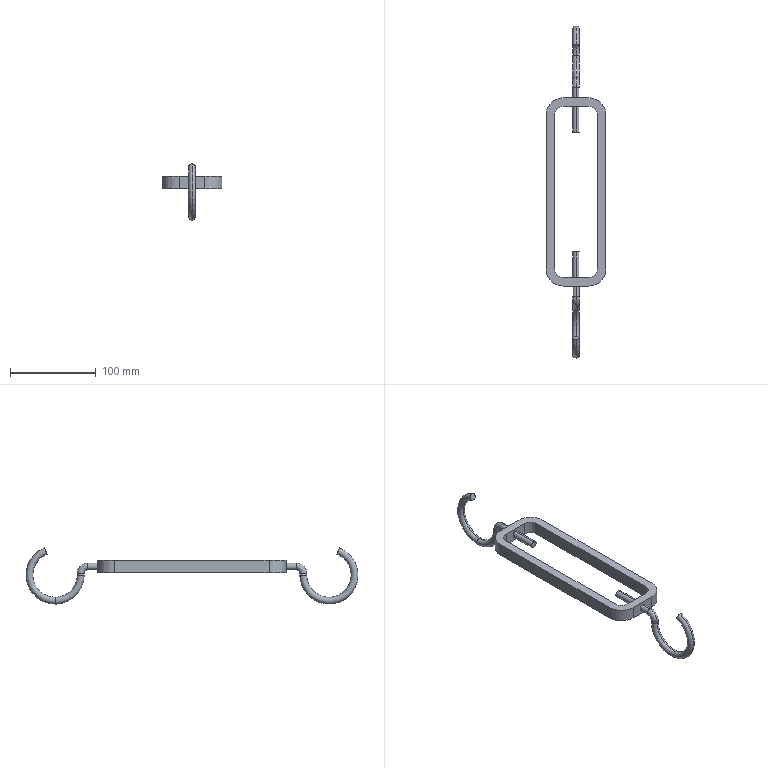Part | SolidWorks | features Extrusion 1, ICE 1, MirrorPattern 1, Sweep 1 | 1 solid | 44 faces | box 70 x 388 x 65.733 mm | volume 95929 mm3 | cylinder 20 | plane 14 | torus 10 | commonest cylinder face diameters 8 x12 20 x4 40 x4
STEP:
#1=CARTESIAN_POINT('',(-4.,-130.,-10.));
#2=VERTEX_POINT('',#1);
#3=CARTESIAN_POINT('',(0.,-126.,-10.));
#4=VERTEX_POINT('',#3);
#5=CARTESIAN_POINT('',(0.,-130.,-10.));
#6=DIRECTION('',(0.,0.,-1.));
#7=DIRECTION('',(0.,-1.,0.));
#8=AXIS2_PLACEMENT_3D('',#5,#6,#7);
#9=CIRCLE('',#8,4.);
#10=EDGE_CURVE('',#2,#4,#9,.T.);
#11=ORIENTED_EDGE('',*,*,#10,.T.);
#12=CARTESIAN_POINT('',(0.,-172.206,21.733));
#13=VERTEX_POINT('',#12);
#14=CARTESIAN_POINT('',(0.,-160.,-10.));
#15=DIRECTION('',(-1.,0.,0.));
#16=DIRECTION('',(0.,0.,1.));
#17=AXIS2_PLACEMENT_3D('',#14,#15,#16);
#18=CIRCLE('',#17,34.);
#19=EDGE_CURVE('',#4,#13,#18,.T.);
#20=ORIENTED_EDGE('',*,*,#19,.T.);
#21=CARTESIAN_POINT('',(0.,-169.334,14.267));
#22=VERTEX_POINT('',#21);
#23=CARTESIAN_POINT('',(0.,-170.77,18.));
#24=DIRECTION('',(0.,0.9333,0.359));
#25=DIRECTION('',(0.,0.359,-0.9333));
#26=AXIS2_PLACEMENT_3D('',#23,#24,#25);
#27=CIRCLE('',#26,4.);
#28=EDGE_CURVE('',#22,#13,#27,.T.);
#29=ORIENTED_EDGE('',*,*,#28,.F.);
#30=CARTESIAN_POINT('',(0.,-134.,-10.));
#31=VERTEX_POINT('',#30);
#32=CARTESIAN_POINT('',(0.,-160.,-10.));
#33=DIRECTION('',(-1.,0.,0.));
#34=DIRECTION('',(0.,0.,1.));
#35=AXIS2_PLACEMENT_3D('',#32,#33,#34);
#36=CIRCLE('',#35,26.);
#37=EDGE_CURVE('',#31,#22,#36,.T.);
#38=ORIENTED_EDGE('',*,*,#37,.F.);
#39=CARTESIAN_POINT('',(0.,-130.,-10.));
#40=DIRECTION('',(0.,0.,-1.));
#41=DIRECTION('',(0.,-1.,0.));
#42=AXIS2_PLACEMENT_3D('',#39,#40,#41);
#43=CIRCLE('',#42,4.);
#44=EDGE_CURVE('',#31,#2,#43,.T.);
#45=ORIENTED_EDGE('',*,*,#44,.T.);
#46=EDGE_LOOP('',(#11,#20,#29,#38,#45));
#47=FACE_OUTER_BOUND('',#46,.T.);
#48=CARTESIAN_POINT('',(0.,-160.,-10.));
#49=DIRECTION('',(-1.,0.,0.));
#50=DIRECTION('',(0.,0.,1.));
#51=AXIS2_PLACEMENT_3D('',#48,#49,#50);
#52=TOROIDAL_SURFACE('',#51,30.,4.);
#53=ADVANCED_FACE('',(#47),#52,.T.);
#54=CARTESIAN_POINT('',(0.,-122.,-4.));
#55=VERTEX_POINT('',#54);
#56=CARTESIAN_POINT('',(0.,-122.,4.));
#57=VERTEX_POINT('',#56);
#58=CARTESIAN_POINT('',(0.,-122.,0.));
#59=DIRECTION('',(0.,-1.,0.));
#60=DIRECTION('',(0.,0.,1.));
#61=AXIS2_PLACEMENT_3D('',#58,#59,#60);
#62=CIRCLE('',#61,4.);
#63=EDGE_CURVE('',#55,#57,#62,.T.);
#64=ORIENTED_EDGE('',*,*,#63,.T.);
#65=CARTESIAN_POINT('',(0.,-134.,-8.));
#66=VERTEX_POINT('',#65);
#67=CARTESIAN_POINT('',(0.,-122.,-8.));
#68=DIRECTION('',(1.,0.,0.));
#69=DIRECTION('',(0.,0.,-1.));
#70=AXIS2_PLACEMENT_3D('',#67,#68,#69);
#71=CIRCLE('',#70,12.);
#72=EDGE_CURVE('',#57,#66,#71,.T.);
#73=ORIENTED_EDGE('',*,*,#72,.T.);
#74=CARTESIAN_POINT('',(4.,-130.,-8.));
#75=VERTEX_POINT('',#74);
#76=CARTESIAN_POINT('',(0.,-130.,-8.));
#77=DIRECTION('',(0.,0.,-1.));
#78=DIRECTION('',(0.,-1.,0.));
#79=AXIS2_PLACEMENT_3D('',#76,#77,#78);
#80=CIRCLE('',#79,4.);
#81=EDGE_CURVE('',#75,#66,#80,.T.);
#82=ORIENTED_EDGE('',*,*,#81,.F.);
#83=CARTESIAN_POINT('',(0.,-126.,-8.));
#84=VERTEX_POINT('',#83);
#85=CARTESIAN_POINT('',(0.,-130.,-8.));
#86=DIRECTION('',(0.,0.,-1.));
#87=DIRECTION('',(0.,-1.,0.));
#88=AXIS2_PLACEMENT_3D('',#85,#86,#87);
#89=CIRCLE('',#88,4.);
#90=EDGE_CURVE('',#84,#75,#89,.T.);
#91=ORIENTED_EDGE('',*,*,#90,.F.);
#92=CARTESIAN_POINT('',(0.,-122.,-8.));
#93=DIRECTION('',(1.,0.,0.));
#94=DIRECTION('',(0.,0.,-1.));
#95=AXIS2_PLACEMENT_3D('',#92,#93,#94);
#96=CIRCLE('',#95,4.);
#97=EDGE_CURVE('',#55,#84,#96,.T.);
#98=ORIENTED_EDGE('',*,*,#97,.F.);
#99=EDGE_LOOP('',(#64,#73,#82,#91,#98));
#100=FACE_OUTER_BOUND('',#99,.T.);
#101=CARTESIAN_POINT('',(0.,-122.,-8.));
#102=DIRECTION('',(1.,0.,0.));
#103=DIRECTION('',(0.,0.,-1.));
#104=AXIS2_PLACEMENT_3D('',#101,#102,#103);
#105=TOROIDAL_SURFACE('',#104,8.,4.);
#106=ADVANCED_FACE('',(#100),#105,.T.);
#107=CARTESIAN_POINT('',(0.,160.,-44.));
#108=VERTEX_POINT('',#107);
#109=CARTESIAN_POINT('',(0.,160.,-36.));
#110=VERTEX_POINT('',#109);
#111=CARTESIAN_POINT('',(0.,160.,-40.));
#112=DIRECTION('',(0.,-1.,0.));
#113=DIRECTION('',(0.,0.,-1.));
#114=AXIS2_PLACEMENT_3D('',#111,#112,#113);
#115=CIRCLE('',#114,4.);
#116=EDGE_CURVE('',#108,#110,#115,.T.);
#117=ORIENTED_EDGE('',*,*,#116,.F.);
#118=CARTESIAN_POINT('',(0.,172.206,21.733));
#119=VERTEX_POINT('',#118);
#120=CARTESIAN_POINT('',(0.,160.,-10.));
#121=DIRECTION('',(1.,0.,0.));
#122=DIRECTION('',(0.,0.,-1.));
#123=AXIS2_PLACEMENT_3D('',#120,#121,#122);
#124=CIRCLE('',#123,34.);
#125=EDGE_CURVE('',#108,#119,#124,.T.);
#126=ORIENTED_EDGE('',*,*,#125,.T.);
#127=CARTESIAN_POINT('',(0.,169.334,14.267));
#128=VERTEX_POINT('',#127);
#129=CARTESIAN_POINT('',(0.,170.77,18.));
#130=DIRECTION('',(0.,-0.9333,0.359));
#131=DIRECTION('',(0.,-0.359,-0.9333));
#132=AXIS2_PLACEMENT_3D('',#129,#130,#131);
#133=CIRCLE('',#132,4.);
#134=EDGE_CURVE('',#128,#119,#133,.T.);
#135=ORIENTED_EDGE('',*,*,#134,.F.);
#136=CARTESIAN_POINT('',(0.,160.,-10.));
#137=DIRECTION('',(1.,0.,0.));
#138=DIRECTION('',(0.,0.,-1.));
#139=AXIS2_PLACEMENT_3D('',#136,#137,#138);
#140=CIRCLE('',#139,26.);
#141=EDGE_CURVE('',#110,#128,#140,.T.);
#142=ORIENTED_EDGE('',*,*,#141,.F.);
#143=EDGE_LOOP('',(#117,#126,#135,#142));
#144=FACE_OUTER_BOUND('',#143,.T.);
#145=CARTESIAN_POINT('',(0.,160.,-10.));
#146=DIRECTION('',(1.,0.,0.));
#147=DIRECTION('',(0.,0.,-1.));
#148=AXIS2_PLACEMENT_3D('',#145,#146,#147);
#149=TOROIDAL_SURFACE('',#148,30.,4.);
#150=ADVANCED_FACE('',(#144),#149,.T.);
#151=CARTESIAN_POINT('',(0.,122.,-4.));
#152=VERTEX_POINT('',#151);
#153=CARTESIAN_POINT('',(0.,122.,4.));
#154=VERTEX_POINT('',#153);
#155=CARTESIAN_POINT('',(0.,122.,0.));
#156=DIRECTION('',(0.,1.,0.));
#157=DIRECTION('',(0.,0.,1.));
#158=AXIS2_PLACEMENT_3D('',#155,#156,#157);
#159=CIRCLE('',#158,4.);
#160=EDGE_CURVE('',#152,#154,#159,.T.);
#161=ORIENTED_EDGE('',*,*,#160,.T.);
#162=CARTESIAN_POINT('',(0.,134.,-8.));
#163=VERTEX_POINT('',#162);
#164=CARTESIAN_POINT('',(0.,122.,-8.));
#165=DIRECTION('',(-1.,0.,0.));
#166=DIRECTION('',(0.,0.,1.));
#167=AXIS2_PLACEMENT_3D('',#164,#165,#166);
#168=CIRCLE('',#167,12.);
#169=EDGE_CURVE('',#154,#163,#168,.T.);
#170=ORIENTED_EDGE('',*,*,#169,.T.);
#171=CARTESIAN_POINT('',(-4.,130.,-8.));
#172=VERTEX_POINT('',#171);
#173=CARTESIAN_POINT('',(0.,130.,-8.));
#174=DIRECTION('',(0.,0.,-1.));
#175=DIRECTION('',(0.,1.,0.));
#176=AXIS2_PLACEMENT_3D('',#173,#174,#175);
#177=CIRCLE('',#176,4.);
#178=EDGE_CURVE('',#172,#163,#177,.T.);
#179=ORIENTED_EDGE('',*,*,#178,.F.);
#180=CARTESIAN_POINT('',(0.,126.,-8.));
#181=VERTEX_POINT('',#180);
#182=CARTESIAN_POINT('',(0.,130.,-8.));
#183=DIRECTION('',(0.,0.,-1.));
#184=DIRECTION('',(0.,1.,0.));
#185=AXIS2_PLACEMENT_3D('',#182,#183,#184);
#186=CIRCLE('',#185,4.);
#187=EDGE_CURVE('',#181,#172,#186,.T.);
#188=ORIENTED_EDGE('',*,*,#187,.F.);
#189=CARTESIAN_POINT('',(0.,122.,-8.));
#190=DIRECTION('',(-1.,0.,0.));
#191=DIRECTION('',(0.,0.,1.));
#192=AXIS2_PLACEMENT_3D('',#189,#190,#191);
#193=CIRCLE('',#192,4.);
#194=EDGE_CURVE('',#152,#181,#193,.T.);
#195=ORIENTED_EDGE('',*,*,#194,.F.);
#196=EDGE_LOOP('',(#161,#170,#179,#188,#195));
#197=FACE_OUTER_BOUND('',#196,.T.);
#198=CARTESIAN_POINT('',(0.,122.,-8.));
#199=DIRECTION('',(-1.,0.,0.));
#200=DIRECTION('',(0.,0.,1.));
#201=AXIS2_PLACEMENT_3D('',#198,#199,#200);
#202=TOROIDAL_SURFACE('',#201,8.,4.);
#203=ADVANCED_FACE('',(#197),#202,.T.);
#204=CARTESIAN_POINT('',(4.,130.,-10.));
#205=VERTEX_POINT('',#204);
#206=CARTESIAN_POINT('',(0.,126.,-10.));
#207=VERTEX_POINT('',#206);
#208=CARTESIAN_POINT('',(0.,130.,-10.));
#209=DIRECTION('',(0.,0.,-1.));
#210=DIRECTION('',(0.,1.,0.));
#211=AXIS2_PLACEMENT_3D('',#208,#209,#210);
#212=CIRCLE('',#211,4.);
#213=EDGE_CURVE('',#205,#207,#212,.T.);
#214=ORIENTED_EDGE('',*,*,#213,.T.);
#215=CARTESIAN_POINT('',(0.,160.,-10.));
#216=DIRECTION('',(1.,0.,0.));
#217=DIRECTION('',(0.,0.,-1.));
#218=AXIS2_PLACEMENT_3D('',#215,#216,#217);
#219=CIRCLE('',#218,34.);
#220=EDGE_CURVE('',#207,#108,#219,.T.);
#221=ORIENTED_EDGE('',*,*,#220,.T.);
#222=ORIENTED_EDGE('',*,*,#116,.T.);
#223=CARTESIAN_POINT('',(0.,134.,-10.));
#224=VERTEX_POINT('',#223);
#225=CARTESIAN_POINT('',(0.,160.,-10.));
#226=DIRECTION('',(1.,0.,0.));
#227=DIRECTION('',(0.,0.,-1.));
#228=AXIS2_PLACEMENT_3D('',#225,#226,#227);
#229=CIRCLE('',#228,26.);
#230=EDGE_CURVE('',#224,#110,#229,.T.);
#231=ORIENTED_EDGE('',*,*,#230,.F.);
#232=CARTESIAN_POINT('',(0.,130.,-10.));
#233=DIRECTION('',(0.,0.,-1.));
#234=DIRECTION('',(0.,1.,0.));
#235=AXIS2_PLACEMENT_3D('',#232,#233,#234);
#236=CIRCLE('',#235,4.);
#237=EDGE_CURVE('',#224,#205,#236,.T.);
#238=ORIENTED_EDGE('',*,*,#237,.T.);
#239=EDGE_LOOP('',(#214,#221,#222,#231,#238));
#240=FACE_OUTER_BOUND('',#239,.T.);
#241=CARTESIAN_POINT('',(0.,160.,-10.));
#242=DIRECTION('',(1.,0.,0.));
#243=DIRECTION('',(0.,0.,-1.));
#244=AXIS2_PLACEMENT_3D('',#241,#242,#243);
#245=TOROIDAL_SURFACE('',#244,30.,4.);
#246=ADVANCED_FACE('',(#240),#245,.T.);
#247=CARTESIAN_POINT('',(0.,-70.,-4.));
#248=VERTEX_POINT('',#247);
#249=CARTESIAN_POINT('',(0.,-70.,4.));
#250=VERTEX_POINT('',#249);
#251=CARTESIAN_POINT('',(0.,-70.,0.));
#252=DIRECTION('',(0.,-1.,0.));
#253=DIRECTION('',(0.,0.,-1.));
#254=AXIS2_PLACEMENT_3D('',#251,#252,#253);
#255=CIRCLE('',#254,4.);
#256=EDGE_CURVE('',#248,#250,#255,.T.);
#257=ORIENTED_EDGE('',*,*,#256,.T.);
#258=CARTESIAN_POINT('',(0.,-100.,4.));
#259=VERTEX_POINT('',#258);
#260=CARTESIAN_POINT('',(0.,-70.,4.));
#261=DIRECTION('',(0.,-1.,0.));
#262=VECTOR('',#261,1000.);
#263=LINE('',#260,#262);
#264=EDGE_CURVE('',#250,#259,#263,.T.);
#265=ORIENTED_EDGE('',*,*,#264,.T.);
#266=CARTESIAN_POINT('',(0.,-100.,-4.));
#267=VERTEX_POINT('',#266);
#268=CARTESIAN_POINT('',(0.,-100.,0.));
#269=DIRECTION('',(0.,1.,0.));
#270=DIRECTION('',(0.,0.,1.));
#271=AXIS2_PLACEMENT_3D('',#268,#269,#270);
#272=CIRCLE('',#271,4.);
#273=EDGE_CURVE('',#259,#267,#272,.T.);
#274=ORIENTED_EDGE('',*,*,#273,.T.);
#275=CARTESIAN_POINT('',(0.,-70.,-4.));
#276=DIRECTION('',(0.,-1.,0.));
#277=VECTOR('',#276,1000.);
#278=LINE('',#275,#277);
#279=EDGE_CURVE('',#248,#267,#278,.T.);
#280=ORIENTED_EDGE('',*,*,#279,.F.);
#281=EDGE_LOOP('',(#257,#265,#274,#280));
#282=FACE_OUTER_BOUND('',#281,.T.);
#283=CARTESIAN_POINT('',(0.,-70.,0.));
#284=DIRECTION('',(0.,-1.,0.));
#285=DIRECTION('',(0.,0.,-1.));
#286=AXIS2_PLACEMENT_3D('',#283,#284,#285);
#287=CYLINDRICAL_SURFACE('',#286,4.);
#288=ADVANCED_FACE('',(#282),#287,.T.);
#289=CARTESIAN_POINT('',(-4.,-130.,-8.));
#290=VERTEX_POINT('',#289);
#291=CARTESIAN_POINT('',(0.,-130.,-8.));
#292=DIRECTION('',(0.,0.,-1.));
#293=DIRECTION('',(0.,-1.,0.));
#294=AXIS2_PLACEMENT_3D('',#291,#292,#293);
#295=CIRCLE('',#294,4.);
#296=EDGE_CURVE('',#290,#84,#295,.T.);
#297=ORIENTED_EDGE('',*,*,#296,.T.);
#298=ORIENTED_EDGE('',*,*,#90,.T.);
#299=CARTESIAN_POINT('',(4.,-130.,-10.));
#300=VERTEX_POINT('',#299);
#301=CARTESIAN_POINT('',(4.,-130.,-8.));
#302=DIRECTION('',(0.,0.,-1.));
#303=VECTOR('',#302,1000.);
#304=LINE('',#301,#303);
#305=EDGE_CURVE('',#75,#300,#304,.T.);
#306=ORIENTED_EDGE('',*,*,#305,.T.);
#307=CARTESIAN_POINT('',(0.,-130.,-10.));
#308=DIRECTION('',(0.,0.,-1.));
#309=DIRECTION('',(0.,-1.,0.));
#310=AXIS2_PLACEMENT_3D('',#307,#308,#309);
#311=CIRCLE('',#310,4.);
#312=EDGE_CURVE('',#4,#300,#311,.T.);
#313=ORIENTED_EDGE('',*,*,#312,.F.);
#314=ORIENTED_EDGE('',*,*,#10,.F.);
#315=CARTESIAN_POINT('',(-4.,-130.,-8.));
#316=DIRECTION('',(0.,0.,-1.));
#317=VECTOR('',#316,1000.);
#318=LINE('',#315,#317);
#319=EDGE_CURVE('',#290,#2,#318,.T.);
#320=ORIENTED_EDGE('',*,*,#319,.F.);
#321=EDGE_LOOP('',(#297,#298,#306,#313,#314,#320));
#322=FACE_OUTER_BOUND('',#321,.T.);
#323=CARTESIAN_POINT('',(0.,-130.,-8.));
#324=DIRECTION('',(0.,0.,-1.));
#325=DIRECTION('',(-1.,0.,0.));
#326=AXIS2_PLACEMENT_3D('',#323,#324,#325);
#327=CYLINDRICAL_SURFACE('',#326,4.);
#328=ADVANCED_FACE('',(#322),#327,.T.);
#329=CARTESIAN_POINT('',(0.,-110.,-4.));
#330=VERTEX_POINT('',#329);
#331=CARTESIAN_POINT('',(0.,-110.,4.));
#332=VERTEX_POINT('',#331);
#333=CARTESIAN_POINT('',(0.,-110.,0.));
#334=DIRECTION('',(0.,-1.,0.));
#335=DIRECTION('',(0.,0.,1.));
#336=AXIS2_PLACEMENT_3D('',#333,#334,#335);
#337=CIRCLE('',#336,4.);
#338=EDGE_CURVE('',#330,#332,#337,.T.);
#339=ORIENTED_EDGE('',*,*,#338,.T.);
#340=CARTESIAN_POINT('',(0.,-110.,4.));
#341=DIRECTION('',(0.,-1.,0.));
#342=VECTOR('',#341,1000.);
#343=LINE('',#340,#342);
#344=EDGE_CURVE('',#332,#57,#343,.T.);
#345=ORIENTED_EDGE('',*,*,#344,.T.);
#346=ORIENTED_EDGE('',*,*,#63,.F.);
#347=CARTESIAN_POINT('',(0.,-110.,-4.));
#348=DIRECTION('',(0.,-1.,0.));
#349=VECTOR('',#348,1000.);
#350=LINE('',#347,#349);
#351=EDGE_CURVE('',#330,#55,#350,.T.);
#352=ORIENTED_EDGE('',*,*,#351,.F.);
#353=EDGE_LOOP('',(#339,#345,#346,#352));
#354=FACE_OUTER_BOUND('',#353,.T.);
#355=CARTESIAN_POINT('',(0.,-110.,0.));
#356=DIRECTION('',(0.,-1.,0.));
#357=DIRECTION('',(0.,0.,-1.));
#358=AXIS2_PLACEMENT_3D('',#355,#356,#357);
#359=CYLINDRICAL_SURFACE('',#358,4.);
#360=ADVANCED_FACE('',(#354),#359,.T.);
#361=CARTESIAN_POINT('',(0.,70.,-4.));
#362=VERTEX_POINT('',#361);
#363=CARTESIAN_POINT('',(0.,70.,4.));
#364=VERTEX_POINT('',#363);
#365=CARTESIAN_POINT('',(0.,70.,0.));
#366=DIRECTION('',(0.,-1.,0.));
#367=DIRECTION('',(0.,0.,-1.));
#368=AXIS2_PLACEMENT_3D('',#365,#366,#367);
#369=CIRCLE('',#368,4.);
#370=EDGE_CURVE('',#362,#364,#369,.T.);
#371=ORIENTED_EDGE('',*,*,#370,.F.);
#372=CARTESIAN_POINT('',(0.,100.,-4.));
#373=VERTEX_POINT('',#372);
#374=CARTESIAN_POINT('',(0.,70.,-4.));
#375=DIRECTION('',(0.,1.,0.));
#376=VECTOR('',#375,1000.);
#377=LINE('',#374,#376);
#378=EDGE_CURVE('',#362,#373,#377,.T.);
#379=ORIENTED_EDGE('',*,*,#378,.T.);
#380=CARTESIAN_POINT('',(0.,100.,4.));
#381=VERTEX_POINT('',#380);
#382=CARTESIAN_POINT('',(0.,100.,0.));
#383=DIRECTION('',(0.,-1.,0.));
#384=DIRECTION('',(0.,0.,-1.));
#385=AXIS2_PLACEMENT_3D('',#382,#383,#384);
#386=CIRCLE('',#385,4.);
#387=EDGE_CURVE('',#373,#381,#386,.T.);
#388=ORIENTED_EDGE('',*,*,#387,.T.);
#389=CARTESIAN_POINT('',(0.,70.,4.));
#390=DIRECTION('',(0.,1.,0.));
#391=VECTOR('',#390,1000.);
#392=LINE('',#389,#391);
#393=EDGE_CURVE('',#364,#381,#392,.T.);
#394=ORIENTED_EDGE('',*,*,#393,.F.);
#395=EDGE_LOOP('',(#371,#379,#388,#394));
#396=FACE_OUTER_BOUND('',#395,.T.);
#397=CARTESIAN_POINT('',(0.,70.,0.));
#398=DIRECTION('',(0.,1.,0.));
#399=DIRECTION('',(0.,0.,1.));
#400=AXIS2_PLACEMENT_3D('',#397,#398,#399);
#401=CYLINDRICAL_SURFACE('',#400,4.);
#402=ADVANCED_FACE('',(#396),#401,.T.);
#403=ORIENTED_EDGE('',*,*,#220,.F.);
#404=CARTESIAN_POINT('',(-4.,130.,-10.));
#405=VERTEX_POINT('',#404);
#406=CARTESIAN_POINT('',(0.,130.,-10.));
#407=DIRECTION('',(0.,0.,-1.));
#408=DIRECTION('',(0.,1.,0.));
#409=AXIS2_PLACEMENT_3D('',#406,#407,#408);
#410=CIRCLE('',#409,4.);
#411=EDGE_CURVE('',#207,#405,#410,.T.);
#412=ORIENTED_EDGE('',*,*,#411,.T.);
#413=CARTESIAN_POINT('',(0.,130.,-10.));
#414=DIRECTION('',(0.,0.,-1.));
#415=DIRECTION('',(0.,1.,0.));
#416=AXIS2_PLACEMENT_3D('',#413,#414,#415);
#417=CIRCLE('',#416,4.);
#418=EDGE_CURVE('',#405,#224,#417,.T.);
#419=ORIENTED_EDGE('',*,*,#418,.T.);
#420=ORIENTED_EDGE('',*,*,#230,.T.);
#421=CARTESIAN_POINT('',(0.,160.,-40.));
#422=DIRECTION('',(0.,-1.,0.));
#423=DIRECTION('',(0.,0.,-1.));
#424=AXIS2_PLACEMENT_3D('',#421,#422,#423);
#425=CIRCLE('',#424,4.);
#426=EDGE_CURVE('',#110,#108,#425,.T.);
#427=ORIENTED_EDGE('',*,*,#426,.T.);
#428=EDGE_LOOP('',(#403,#412,#419,#420,#427));
#429=FACE_OUTER_BOUND('',#428,.T.);
#430=CARTESIAN_POINT('',(0.,160.,-10.));
#431=DIRECTION('',(1.,0.,0.));
#432=DIRECTION('',(0.,0.,-1.));
#433=AXIS2_PLACEMENT_3D('',#430,#431,#432);
#434=TOROIDAL_SURFACE('',#433,30.,4.);
#435=ADVANCED_FACE('',(#429),#434,.T.);
#436=ORIENTED_EDGE('',*,*,#178,.T.);
#437=CARTESIAN_POINT('',(4.,130.,-8.));
#438=VERTEX_POINT('',#437);
#439=CARTESIAN_POINT('',(0.,130.,-8.));
#440=DIRECTION('',(0.,0.,-1.));
#441=DIRECTION('',(0.,1.,0.));
#442=AXIS2_PLACEMENT_3D('',#439,#440,#441);
#443=CIRCLE('',#442,4.);
#444=EDGE_CURVE('',#163,#438,#443,.T.);
#445=ORIENTED_EDGE('',*,*,#444,.T.);
#446=CARTESIAN_POINT('',(4.,130.,-8.));
#447=DIRECTION('',(0.,0.,-1.));
#448=VECTOR('',#447,1000.);
#449=LINE('',#446,#448);
#450=EDGE_CURVE('',#438,#205,#449,.T.);
#451=ORIENTED_EDGE('',*,*,#450,.T.);
#452=ORIENTED_EDGE('',*,*,#237,.F.);
#453=ORIENTED_EDGE('',*,*,#418,.F.);
#454=CARTESIAN_POINT('',(-4.,130.,-8.));
#455=DIRECTION('',(0.,0.,-1.));
#456=VECTOR('',#455,1000.);
#457=LINE('',#454,#456);
#458=EDGE_CURVE('',#172,#405,#457,.T.);
#459=ORIENTED_EDGE('',*,*,#458,.F.);
#460=EDGE_LOOP('',(#436,#445,#451,#452,#453,#459));
#461=FACE_OUTER_BOUND('',#460,.T.);
#462=CARTESIAN_POINT('',(0.,130.,-8.));
#463=DIRECTION('',(0.,0.,-1.));
#464=DIRECTION('',(-1.,0.,0.));
#465=AXIS2_PLACEMENT_3D('',#462,#463,#464);
#466=CYLINDRICAL_SURFACE('',#465,4.);
#467=ADVANCED_FACE('',(#461),#466,.T.);
#468=CARTESIAN_POINT('',(0.,110.,4.));
#469=VERTEX_POINT('',#468);
#470=CARTESIAN_POINT('',(0.,110.,-4.));
#471=VERTEX_POINT('',#470);
#472=CARTESIAN_POINT('',(0.,110.,0.));
#473=DIRECTION('',(0.,1.,0.));
#474=DIRECTION('',(0.,0.,1.));
#475=AXIS2_PLACEMENT_3D('',#472,#473,#474);
#476=CIRCLE('',#475,4.);
#477=EDGE_CURVE('',#469,#471,#476,.T.);
#478=ORIENTED_EDGE('',*,*,#477,.T.);
#479=CARTESIAN_POINT('',(0.,110.,-4.));
#480=DIRECTION('',(0.,1.,0.));
#481=VECTOR('',#480,1000.);
#482=LINE('',#479,#481);
#483=EDGE_CURVE('',#471,#152,#482,.T.);
#484=ORIENTED_EDGE('',*,*,#483,.T.);
#485=CARTESIAN_POINT('',(0.,122.,0.));
#486=DIRECTION('',(0.,1.,0.));
#487=DIRECTION('',(0.,0.,1.));
#488=AXIS2_PLACEMENT_3D('',#485,#486,#487);
#489=CIRCLE('',#488,4.);
#490=EDGE_CURVE('',#154,#152,#489,.T.);
#491=ORIENTED_EDGE('',*,*,#490,.F.);
#492=CARTESIAN_POINT('',(0.,110.,4.));
#493=DIRECTION('',(0.,1.,0.));
#494=VECTOR('',#493,1000.);
#495=LINE('',#492,#494);
#496=EDGE_CURVE('',#469,#154,#495,.T.);
#497=ORIENTED_EDGE('',*,*,#496,.F.);
#498=EDGE_LOOP('',(#478,#484,#491,#497));
#499=FACE_OUTER_BOUND('',#498,.T.);
#500=CARTESIAN_POINT('',(0.,110.,0.));
#501=DIRECTION('',(0.,1.,0.));
#502=DIRECTION('',(0.,0.,1.));
#503=AXIS2_PLACEMENT_3D('',#500,#501,#502);
#504=CYLINDRICAL_SURFACE('',#503,4.);
#505=ADVANCED_FACE('',(#499),#504,.T.);
#506=CARTESIAN_POINT('',(-15.,110.,7.5));
#507=VERTEX_POINT('',#506);
#508=CARTESIAN_POINT('',(-35.,90.,7.5));
#509=VERTEX_POINT('',#508);
#510=CARTESIAN_POINT('',(-15.,90.,7.5));
#511=DIRECTION('',(0.,0.,1.));
#512=DIRECTION('',(-1.,0.,0.));
#513=AXIS2_PLACEMENT_3D('',#510,#511,#512);
#514=CIRCLE('',#513,20.);
#515=EDGE_CURVE('',#507,#509,#514,.T.);
#516=ORIENTED_EDGE('',*,*,#515,.T.);
#517=CARTESIAN_POINT('',(-35.,-90.,7.5));
#518=VERTEX_POINT('',#517);
#519=CARTESIAN_POINT('',(-35.,-90.,7.5));
#520=DIRECTION('',(0.,-1.,0.));
#521=VECTOR('',#520,1000.);
#522=LINE('',#519,#521);
#523=EDGE_CURVE('',#509,#518,#522,.T.);
#524=ORIENTED_EDGE('',*,*,#523,.T.);
#525=CARTESIAN_POINT('',(-15.,-110.,7.5));
#526=VERTEX_POINT('',#525);
#527=CARTESIAN_POINT('',(-15.,-90.,7.5));
#528=DIRECTION('',(0.,0.,1.));
#529=DIRECTION('',(-1.,0.,0.));
#530=AXIS2_PLACEMENT_3D('',#527,#528,#529);
#531=CIRCLE('',#530,20.);
#532=EDGE_CURVE('',#518,#526,#531,.T.);
#533=ORIENTED_EDGE('',*,*,#532,.T.);
#534=CARTESIAN_POINT('',(15.,-110.,7.5));
#535=VERTEX_POINT('',#534);
#536=CARTESIAN_POINT('',(-15.,-110.,7.5));
#537=DIRECTION('',(1.,0.,0.));
#538=VECTOR('',#537,1000.);
#539=LINE('',#536,#538);
#540=EDGE_CURVE('',#526,#535,#539,.T.);
#541=ORIENTED_EDGE('',*,*,#540,.T.);
#542=CARTESIAN_POINT('',(35.,-90.,7.5));
#543=VERTEX_POINT('',#542);
#544=CARTESIAN_POINT('',(15.,-90.,7.5));
#545=DIRECTION('',(0.,0.,1.));
#546=DIRECTION('',(1.,0.,0.));
#547=AXIS2_PLACEMENT_3D('',#544,#545,#546);
#548=CIRCLE('',#547,20.);
#549=EDGE_CURVE('',#535,#543,#548,.T.);
#550=ORIENTED_EDGE('',*,*,#549,.T.);
#551=CARTESIAN_POINT('',(35.,90.,7.5));
#552=VERTEX_POINT('',#551);
#553=CARTESIAN_POINT('',(35.,-90.,7.5));
#554=DIRECTION('',(0.,1.,0.));
#555=VECTOR('',#554,1000.);
#556=LINE('',#553,#555);
#557=EDGE_CURVE('',#543,#552,#556,.T.);
#558=ORIENTED_EDGE('',*,*,#557,.T.);
#559=CARTESIAN_POINT('',(15.,110.,7.5));
#560=VERTEX_POINT('',#559);
#561=CARTESIAN_POINT('',(15.,90.,7.5));
#562=DIRECTION('',(0.,0.,1.));
#563=DIRECTION('',(-1.,0.,0.));
#564=AXIS2_PLACEMENT_3D('',#561,#562,#563);
#565=CIRCLE('',#564,20.);
#566=EDGE_CURVE('',#552,#560,#565,.T.);
#567=ORIENTED_EDGE('',*,*,#566,.T.);
#568=CARTESIAN_POINT('',(-15.,110.,7.5));
#569=DIRECTION('',(-1.,0.,0.));
#570=VECTOR('',#569,1000.);
#571=LINE('',#568,#570);
#572=EDGE_CURVE('',#560,#507,#571,.T.);
#573=ORIENTED_EDGE('',*,*,#572,.T.);
#574=EDGE_LOOP('',(#516,#524,#533,#541,#550,#558,#567,#573));
#575=FACE_OUTER_BOUND('',#574,.T.);
#576=CARTESIAN_POINT('',(15.,-100.,7.5));
#577=VERTEX_POINT('',#576);
#578=CARTESIAN_POINT('',(25.,-90.,7.5));
#579=VERTEX_POINT('',#578);
#580=CARTESIAN_POINT('',(15.,-90.,7.5));
#581=DIRECTION('',(0.,0.,1.));
#582=DIRECTION('',(1.,0.,0.));
#583=AXIS2_PLACEMENT_3D('',#580,#581,#582);
#584=CIRCLE('',#583,10.);
#585=EDGE_CURVE('',#577,#579,#584,.T.);
#586=ORIENTED_EDGE('',*,*,#585,.F.);
#587=CARTESIAN_POINT('',(-15.,-100.,7.5));
#588=VERTEX_POINT('',#587);
#589=CARTESIAN_POINT('',(-15.,-100.,7.5));
#590=DIRECTION('',(1.,0.,0.));
#591=VECTOR('',#590,1000.);
#592=LINE('',#589,#591);
#593=EDGE_CURVE('',#588,#577,#592,.T.);
#594=ORIENTED_EDGE('',*,*,#593,.F.);
#595=CARTESIAN_POINT('',(-25.,-90.,7.5));
#596=VERTEX_POINT('',#595);
#597=CARTESIAN_POINT('',(-15.,-90.,7.5));
#598=DIRECTION('',(0.,0.,1.));
#599=DIRECTION('',(-1.,0.,0.));
#600=AXIS2_PLACEMENT_3D('',#597,#598,#599);
#601=CIRCLE('',#600,10.);
#602=EDGE_CURVE('',#596,#588,#601,.T.);
#603=ORIENTED_EDGE('',*,*,#602,.F.);
#604=CARTESIAN_POINT('',(-25.,90.,7.5));
#605=VERTEX_POINT('',#604);
#606=CARTESIAN_POINT('',(-25.,-90.,7.5));
#607=DIRECTION('',(0.,-1.,0.));
#608=VECTOR('',#607,1000.);
#609=LINE('',#606,#608);
#610=EDGE_CURVE('',#605,#596,#609,.T.);
#611=ORIENTED_EDGE('',*,*,#610,.F.);
#612=CARTESIAN_POINT('',(-15.,100.,7.5));
#613=VERTEX_POINT('',#612);
#614=CARTESIAN_POINT('',(-15.,90.,7.5));
#615=DIRECTION('',(0.,0.,1.));
#616=DIRECTION('',(-1.,0.,0.));
#617=AXIS2_PLACEMENT_3D('',#614,#615,#616);
#618=CIRCLE('',#617,10.);
#619=EDGE_CURVE('',#613,#605,#618,.T.);
#620=ORIENTED_EDGE('',*,*,#619,.F.);
#621=CARTESIAN_POINT('',(15.,100.,7.5));
#622=VERTEX_POINT('',#621);
#623=CARTESIAN_POINT('',(-15.,100.,7.5));
#624=DIRECTION('',(-1.,0.,0.));
#625=VECTOR('',#624,1000.);
#626=LINE('',#623,#625);
#627=EDGE_CURVE('',#622,#613,#626,.T.);
#628=ORIENTED_EDGE('',*,*,#627,.F.);
#629=CARTESIAN_POINT('',(25.,90.,7.5));
#630=VERTEX_POINT('',#629);
#631=CARTESIAN_POINT('',(15.,90.,7.5));
#632=DIRECTION('',(0.,0.,1.));
#633=DIRECTION('',(-1.,0.,0.));
#634=AXIS2_PLACEMENT_3D('',#631,#632,#633);
#635=CIRCLE('',#634,10.);
#636=EDGE_CURVE('',#630,#622,#635,.T.);
#637=ORIENTED_EDGE('',*,*,#636,.F.);
#638=CARTESIAN_POINT('',(25.,-90.,7.5));
#639=DIRECTION('',(0.,1.,0.));
#640=VECTOR('',#639,1000.);
#641=LINE('',#638,#640);
#642=EDGE_CURVE('',#579,#630,#641,.T.);
#643=ORIENTED_EDGE('',*,*,#642,.F.);
#644=EDGE_LOOP('',(#586,#594,#603,#611,#620,#628,#637,#643));
#645=FACE_BOUND('',#644,.T.);
#646=CARTESIAN_POINT('',(-15.,90.,7.5));
#647=DIRECTION('',(0.,0.,-1.));
#648=DIRECTION('',(-1.,0.,0.));
#649=AXIS2_PLACEMENT_3D('',#646,#647,#648);
#650=PLANE('',#649);
#651=ADVANCED_FACE('',(#575,#645),#650,.F.);
#652=CARTESIAN_POINT('',(-15.,110.,-7.5));
#653=VERTEX_POINT('',#652);
#654=CARTESIAN_POINT('',(-35.,90.,-7.5));
#655=VERTEX_POINT('',#654);
#656=CARTESIAN_POINT('',(-15.,90.,-7.5));
#657=DIRECTION('',(0.,0.,1.));
#658=DIRECTION('',(-1.,0.,0.));
#659=AXIS2_PLACEMENT_3D('',#656,#657,#658);
#660=CIRCLE('',#659,20.);
#661=EDGE_CURVE('',#653,#655,#660,.T.);
#662=ORIENTED_EDGE('',*,*,#661,.F.);
#663=CARTESIAN_POINT('',(15.,110.,-7.5));
#664=VERTEX_POINT('',#663);
#665=CARTESIAN_POINT('',(-15.,110.,-7.5));
#666=DIRECTION('',(-1.,0.,0.));
#667=VECTOR('',#666,1000.);
#668=LINE('',#665,#667);
#669=EDGE_CURVE('',#664,#653,#668,.T.);
#670=ORIENTED_EDGE('',*,*,#669,.F.);
#671=CARTESIAN_POINT('',(35.,90.,-7.5));
#672=VERTEX_POINT('',#671);
#673=CARTESIAN_POINT('',(15.,90.,-7.5));
#674=DIRECTION('',(0.,0.,1.));
#675=DIRECTION('',(-1.,0.,0.));
#676=AXIS2_PLACEMENT_3D('',#673,#674,#675);
#677=CIRCLE('',#676,20.);
#678=EDGE_CURVE('',#672,#664,#677,.T.);
#679=ORIENTED_EDGE('',*,*,#678,.F.);
#680=CARTESIAN_POINT('',(35.,-90.,-7.5));
#681=VERTEX_POINT('',#680);
#682=CARTESIAN_POINT('',(35.,-90.,-7.5));
#683=DIRECTION('',(0.,1.,0.));
#684=VECTOR('',#683,1000.);
#685=LINE('',#682,#684);
#686=EDGE_CURVE('',#681,#672,#685,.T.);
#687=ORIENTED_EDGE('',*,*,#686,.F.);
#688=CARTESIAN_POINT('',(15.,-110.,-7.5));
#689=VERTEX_POINT('',#688);
#690=CARTESIAN_POINT('',(15.,-90.,-7.5));
#691=DIRECTION('',(0.,0.,1.));
#692=DIRECTION('',(1.,0.,0.));
#693=AXIS2_PLACEMENT_3D('',#690,#691,#692);
#694=CIRCLE('',#693,20.);
#695=EDGE_CURVE('',#689,#681,#694,.T.);
#696=ORIENTED_EDGE('',*,*,#695,.F.);
#697=CARTESIAN_POINT('',(-15.,-110.,-7.5));
#698=VERTEX_POINT('',#697);
#699=CARTESIAN_POINT('',(-15.,-110.,-7.5));
#700=DIRECTION('',(1.,0.,0.));
#701=VECTOR('',#700,1000.);
#702=LINE('',#699,#701);
#703=EDGE_CURVE('',#698,#689,#702,.T.);
#704=ORIENTED_EDGE('',*,*,#703,.F.);
#705=CARTESIAN_POINT('',(-35.,-90.,-7.5));
#706=VERTEX_POINT('',#705);
#707=CARTESIAN_POINT('',(-15.,-90.,-7.5));
#708=DIRECTION('',(0.,0.,1.));
#709=DIRECTION('',(-1.,0.,0.));
#710=AXIS2_PLACEMENT_3D('',#707,#708,#709);
#711=CIRCLE('',#710,20.);
#712=EDGE_CURVE('',#706,#698,#711,.T.);
#713=ORIENTED_EDGE('',*,*,#712,.F.);
#714=CARTESIAN_POINT('',(-35.,-90.,-7.5));
#715=DIRECTION('',(0.,-1.,0.));
#716=VECTOR('',#715,1000.);
#717=LINE('',#714,#716);
#718=EDGE_CURVE('',#655,#706,#717,.T.);
#719=ORIENTED_EDGE('',*,*,#718,.F.);
#720=EDGE_LOOP('',(#662,#670,#679,#687,#696,#704,#713,#719));
#721=FACE_OUTER_BOUND('',#720,.T.);
#722=CARTESIAN_POINT('',(-15.,-100.,-7.5));
#723=VERTEX_POINT('',#722);
#724=CARTESIAN_POINT('',(15.,-100.,-7.5));
#725=VERTEX_POINT('',#724);
#726=CARTESIAN_POINT('',(-15.,-100.,-7.5));
#727=DIRECTION('',(1.,0.,0.));
#728=VECTOR('',#727,1000.);
#729=LINE('',#726,#728);
#730=EDGE_CURVE('',#723,#725,#729,.T.);
#731=ORIENTED_EDGE('',*,*,#730,.T.);
#732=CARTESIAN_POINT('',(25.,-90.,-7.5));
#733=VERTEX_POINT('',#732);
#734=CARTESIAN_POINT('',(15.,-90.,-7.5));
#735=DIRECTION('',(0.,0.,1.));
#736=DIRECTION('',(1.,0.,0.));
#737=AXIS2_PLACEMENT_3D('',#734,#735,#736);
#738=CIRCLE('',#737,10.);
#739=EDGE_CURVE('',#725,#733,#738,.T.);
#740=ORIENTED_EDGE('',*,*,#739,.T.);
#741=CARTESIAN_POINT('',(25.,90.,-7.5));
#742=VERTEX_POINT('',#741);
#743=CARTESIAN_POINT('',(25.,-90.,-7.5));
#744=DIRECTION('',(0.,1.,0.));
#745=VECTOR('',#744,1000.);
#746=LINE('',#743,#745);
#747=EDGE_CURVE('',#733,#742,#746,.T.);
#748=ORIENTED_EDGE('',*,*,#747,.T.);
#749=CARTESIAN_POINT('',(15.,100.,-7.5));
#750=VERTEX_POINT('',#749);
#751=CARTESIAN_POINT('',(15.,90.,-7.5));
#752=DIRECTION('',(0.,0.,1.));
#753=DIRECTION('',(-1.,0.,0.));
#754=AXIS2_PLACEMENT_3D('',#751,#752,#753);
#755=CIRCLE('',#754,10.);
#756=EDGE_CURVE('',#742,#750,#755,.T.);
#757=ORIENTED_EDGE('',*,*,#756,.T.);
#758=CARTESIAN_POINT('',(-15.,100.,-7.5));
#759=VERTEX_POINT('',#758);
#760=CARTESIAN_POINT('',(-15.,100.,-7.5));
#761=DIRECTION('',(-1.,0.,0.));
#762=VECTOR('',#761,1000.);
#763=LINE('',#760,#762);
#764=EDGE_CURVE('',#750,#759,#763,.T.);
#765=ORIENTED_EDGE('',*,*,#764,.T.);
#766=CARTESIAN_POINT('',(-25.,90.,-7.5));
#767=VERTEX_POINT('',#766);
#768=CARTESIAN_POINT('',(-15.,90.,-7.5));
#769=DIRECTION('',(0.,0.,1.));
#770=DIRECTION('',(-1.,0.,0.));
#771=AXIS2_PLACEMENT_3D('',#768,#769,#770);
#772=CIRCLE('',#771,10.);
#773=EDGE_CURVE('',#759,#767,#772,.T.);
#774=ORIENTED_EDGE('',*,*,#773,.T.);
#775=CARTESIAN_POINT('',(-25.,-90.,-7.5));
#776=VERTEX_POINT('',#775);
#777=CARTESIAN_POINT('',(-25.,-90.,-7.5));
#778=DIRECTION('',(0.,-1.,0.));
#779=VECTOR('',#778,1000.);
#780=LINE('',#777,#779);
#781=EDGE_CURVE('',#767,#776,#780,.T.);
#782=ORIENTED_EDGE('',*,*,#781,.T.);
#783=CARTESIAN_POINT('',(-15.,-90.,-7.5));
#784=DIRECTION('',(0.,0.,1.));
#785=DIRECTION('',(-1.,0.,0.));
#786=AXIS2_PLACEMENT_3D('',#783,#784,#785);
#787=CIRCLE('',#786,10.);
#788=EDGE_CURVE('',#776,#723,#787,.T.);
#789=ORIENTED_EDGE('',*,*,#788,.T.);
#790=EDGE_LOOP('',(#731,#740,#748,#757,#765,#774,#782,#789));
#791=FACE_BOUND('',#790,.T.);
#792=CARTESIAN_POINT('',(-15.,90.,-7.5));
#793=DIRECTION('',(0.,0.,-1.));
#794=DIRECTION('',(-1.,0.,0.));
#795=AXIS2_PLACEMENT_3D('',#792,#793,#794);
#796=PLANE('',#795);
#797=ADVANCED_FACE('',(#721,#791),#796,.T.);
#798=ORIENTED_EDGE('',*,*,#661,.T.);
#799=CARTESIAN_POINT('',(-35.,90.,7.5));
#800=DIRECTION('',(0.,0.,-1.));
#801=VECTOR('',#800,1000.);
#802=LINE('',#799,#801);
#803=EDGE_CURVE('',#509,#655,#802,.T.);
#804=ORIENTED_EDGE('',*,*,#803,.F.);
#805=ORIENTED_EDGE('',*,*,#515,.F.);
#806=CARTESIAN_POINT('',(-15.,110.,7.5));
#807=DIRECTION('',(0.,0.,-1.));
#808=VECTOR('',#807,1000.);
#809=LINE('',#806,#808);
#810=EDGE_CURVE('',#507,#653,#809,.T.);
#811=ORIENTED_EDGE('',*,*,#810,.T.);
#812=EDGE_LOOP('',(#798,#804,#805,#811));
#813=FACE_OUTER_BOUND('',#812,.T.);
#814=CARTESIAN_POINT('',(-15.,90.,7.5));
#815=DIRECTION('',(0.,0.,-1.));
#816=DIRECTION('',(-1.,0.,0.));
#817=AXIS2_PLACEMENT_3D('',#814,#815,#816);
#818=CYLINDRICAL_SURFACE('',#817,20.);
#819=ADVANCED_FACE('',(#813),#818,.T.);
#820=ORIENTED_EDGE('',*,*,#718,.T.);
#821=CARTESIAN_POINT('',(-35.,-90.,7.5));
#822=DIRECTION('',(0.,0.,-1.));
#823=VECTOR('',#822,1000.);
#824=LINE('',#821,#823);
#825=EDGE_CURVE('',#518,#706,#824,.T.);
#826=ORIENTED_EDGE('',*,*,#825,.F.);
#827=ORIENTED_EDGE('',*,*,#523,.F.);
#828=ORIENTED_EDGE('',*,*,#803,.T.);
#829=EDGE_LOOP('',(#820,#826,#827,#828));
#830=FACE_OUTER_BOUND('',#829,.T.);
#831=CARTESIAN_POINT('',(-35.,-90.,7.5));
#832=DIRECTION('',(1.,0.,0.));
#833=DIRECTION('',(0.,0.,-1.));
#834=AXIS2_PLACEMENT_3D('',#831,#832,#833);
#835=PLANE('',#834);
#836=ADVANCED_FACE('',(#830),#835,.F.);
#837=ORIENTED_EDGE('',*,*,#712,.T.);
#838=CARTESIAN_POINT('',(-15.,-110.,7.5));
#839=DIRECTION('',(0.,0.,-1.));
#840=VECTOR('',#839,1000.);
#841=LINE('',#838,#840);
#842=EDGE_CURVE('',#526,#698,#841,.T.);
#843=ORIENTED_EDGE('',*,*,#842,.F.);
#844=ORIENTED_EDGE('',*,*,#532,.F.);
#845=ORIENTED_EDGE('',*,*,#825,.T.);
#846=EDGE_LOOP('',(#837,#843,#844,#845));
#847=FACE_OUTER_BOUND('',#846,.T.);
#848=CARTESIAN_POINT('',(-15.,-90.,7.5));
#849=DIRECTION('',(0.,0.,-1.));
#850=DIRECTION('',(-1.,0.,0.));
#851=AXIS2_PLACEMENT_3D('',#848,#849,#850);
#852=CYLINDRICAL_SURFACE('',#851,20.);
#853=ADVANCED_FACE('',(#847),#852,.T.);
#854=ORIENTED_EDGE('',*,*,#338,.F.);
#855=CARTESIAN_POINT('',(0.,-110.,0.));
#856=DIRECTION('',(0.,-1.,0.));
#857=DIRECTION('',(0.,0.,1.));
#858=AXIS2_PLACEMENT_3D('',#855,#856,#857);
#859=CIRCLE('',#858,4.);
#860=EDGE_CURVE('',#332,#330,#859,.T.);
#861=ORIENTED_EDGE('',*,*,#860,.F.);
#862=EDGE_LOOP('',(#854,#861));
#863=FACE_BOUND('',#862,.T.);
#864=ORIENTED_EDGE('',*,*,#703,.T.);
#865=CARTESIAN_POINT('',(15.,-110.,7.5));
#866=DIRECTION('',(0.,0.,-1.));
#867=VECTOR('',#866,1000.);
#868=LINE('',#865,#867);
#869=EDGE_CURVE('',#535,#689,#868,.T.);
#870=ORIENTED_EDGE('',*,*,#869,.F.);
#871=ORIENTED_EDGE('',*,*,#540,.F.);
#872=ORIENTED_EDGE('',*,*,#842,.T.);
#873=EDGE_LOOP('',(#864,#870,#871,#872));
#874=FACE_OUTER_BOUND('',#873,.T.);
#875=CARTESIAN_POINT('',(-15.,-110.,7.5));
#876=DIRECTION('',(0.,1.,0.));
#877=DIRECTION('',(-1.,0.,0.));
#878=AXIS2_PLACEMENT_3D('',#875,#876,#877);
#879=PLANE('',#878);
#880=ADVANCED_FACE('',(#863,#874),#879,.F.);
#881=ORIENTED_EDGE('',*,*,#695,.T.);
#882=CARTESIAN_POINT('',(35.,-90.,7.5));
#883=DIRECTION('',(0.,0.,-1.));
#884=VECTOR('',#883,1000.);
#885=LINE('',#882,#884);
#886=EDGE_CURVE('',#543,#681,#885,.T.);
#887=ORIENTED_EDGE('',*,*,#886,.F.);
#888=ORIENTED_EDGE('',*,*,#549,.F.);
#889=ORIENTED_EDGE('',*,*,#869,.T.);
#890=EDGE_LOOP('',(#881,#887,#888,#889));
#891=FACE_OUTER_BOUND('',#890,.T.);
#892=CARTESIAN_POINT('',(15.,-90.,7.5));
#893=DIRECTION('',(0.,0.,-1.));
#894=DIRECTION('',(-1.,0.,0.));
#895=AXIS2_PLACEMENT_3D('',#892,#893,#894);
#896=CYLINDRICAL_SURFACE('',#895,20.);
#897=ADVANCED_FACE('',(#891),#896,.T.);
#898=ORIENTED_EDGE('',*,*,#686,.T.);
#899=CARTESIAN_POINT('',(35.,90.,7.5));
#900=DIRECTION('',(0.,0.,-1.));
#901=VECTOR('',#900,1000.);
#902=LINE('',#899,#901);
#903=EDGE_CURVE('',#552,#672,#902,.T.);
#904=ORIENTED_EDGE('',*,*,#903,.F.);
#905=ORIENTED_EDGE('',*,*,#557,.F.);
#906=ORIENTED_EDGE('',*,*,#886,.T.);
#907=EDGE_LOOP('',(#898,#904,#905,#906));
#908=FACE_OUTER_BOUND('',#907,.T.);
#909=CARTESIAN_POINT('',(35.,-90.,7.5));
#910=DIRECTION('',(-1.,0.,0.));
#911=DIRECTION('',(0.,0.,1.));
#912=AXIS2_PLACEMENT_3D('',#909,#910,#911);
#913=PLANE('',#912);
#914=ADVANCED_FACE('',(#908),#913,.F.);
#915=ORIENTED_EDGE('',*,*,#678,.T.);
#916=CARTESIAN_POINT('',(15.,110.,7.5));
#917=DIRECTION('',(0.,0.,-1.));
#918=VECTOR('',#917,1000.);
#919=LINE('',#916,#918);
#920=EDGE_CURVE('',#560,#664,#919,.T.);
#921=ORIENTED_EDGE('',*,*,#920,.F.);
#922=ORIENTED_EDGE('',*,*,#566,.F.);
#923=ORIENTED_EDGE('',*,*,#903,.T.);
#924=EDGE_LOOP('',(#915,#921,#922,#923));
#925=FACE_OUTER_BOUND('',#924,.T.);
#926=CARTESIAN_POINT('',(15.,90.,7.5));
#927=DIRECTION('',(0.,0.,-1.));
#928=DIRECTION('',(-1.,0.,0.));
#929=AXIS2_PLACEMENT_3D('',#926,#927,#928);
#930=CYLINDRICAL_SURFACE('',#929,20.);
#931=ADVANCED_FACE('',(#925),#930,.T.);
#932=ORIENTED_EDGE('',*,*,#477,.F.);
#933=CARTESIAN_POINT('',(0.,110.,0.));
#934=DIRECTION('',(0.,1.,0.));
#935=DIRECTION('',(0.,0.,1.));
#936=AXIS2_PLACEMENT_3D('',#933,#934,#935);
#937=CIRCLE('',#936,4.);
#938=EDGE_CURVE('',#471,#469,#937,.T.);
#939=ORIENTED_EDGE('',*,*,#938,.F.);
#940=EDGE_LOOP('',(#932,#939));
#941=FACE_BOUND('',#940,.T.);
#942=ORIENTED_EDGE('',*,*,#669,.T.);
#943=ORIENTED_EDGE('',*,*,#810,.F.);
#944=ORIENTED_EDGE('',*,*,#572,.F.);
#945=ORIENTED_EDGE('',*,*,#920,.T.);
#946=EDGE_LOOP('',(#942,#943,#944,#945));
#947=FACE_OUTER_BOUND('',#946,.T.);
#948=CARTESIAN_POINT('',(-15.,110.,7.5));
#949=DIRECTION('',(0.,-1.,0.));
#950=DIRECTION('',(0.,0.,-1.));
#951=AXIS2_PLACEMENT_3D('',#948,#949,#950);
#952=PLANE('',#951);
#953=ADVANCED_FACE('',(#941,#947),#952,.F.);
#954=ORIENTED_EDGE('',*,*,#739,.F.);
#955=CARTESIAN_POINT('',(15.,-100.,7.5));
#956=DIRECTION('',(0.,0.,-1.));
#957=VECTOR('',#956,1000.);
#958=LINE('',#955,#957);
#959=EDGE_CURVE('',#577,#725,#958,.T.);
#960=ORIENTED_EDGE('',*,*,#959,.F.);
#961=ORIENTED_EDGE('',*,*,#585,.T.);
#962=CARTESIAN_POINT('',(25.,-90.,7.5));
#963=DIRECTION('',(0.,0.,-1.));
#964=VECTOR('',#963,1000.);
#965=LINE('',#962,#964);
#966=EDGE_CURVE('',#579,#733,#965,.T.);
#967=ORIENTED_EDGE('',*,*,#966,.T.);
#968=EDGE_LOOP('',(#954,#960,#961,#967));
#969=FACE_OUTER_BOUND('',#968,.T.);
#970=CARTESIAN_POINT('',(15.,-90.,7.5));
#971=DIRECTION('',(0.,0.,-1.));
#972=DIRECTION('',(-1.,0.,0.));
#973=AXIS2_PLACEMENT_3D('',#970,#971,#972);
#974=CYLINDRICAL_SURFACE('',#973,10.);
#975=ADVANCED_FACE('',(#969),#974,.F.);
#976=ORIENTED_EDGE('',*,*,#747,.F.);
#977=ORIENTED_EDGE('',*,*,#966,.F.);
#978=ORIENTED_EDGE('',*,*,#642,.T.);
#979=CARTESIAN_POINT('',(25.,90.,7.5));
#980=DIRECTION('',(0.,0.,-1.));
#981=VECTOR('',#980,1000.);
#982=LINE('',#979,#981);
#983=EDGE_CURVE('',#630,#742,#982,.T.);
#984=ORIENTED_EDGE('',*,*,#983,.T.);
#985=EDGE_LOOP('',(#976,#977,#978,#984));
#986=FACE_OUTER_BOUND('',#985,.T.);
#987=CARTESIAN_POINT('',(25.,-90.,7.5));
#988=DIRECTION('',(-1.,0.,0.));
#989=DIRECTION('',(0.,0.,1.));
#990=AXIS2_PLACEMENT_3D('',#987,#988,#989);
#991=PLANE('',#990);
#992=ADVANCED_FACE('',(#986),#991,.T.);
#993=ORIENTED_EDGE('',*,*,#756,.F.);
#994=ORIENTED_EDGE('',*,*,#983,.F.);
#995=ORIENTED_EDGE('',*,*,#636,.T.);
#996=CARTESIAN_POINT('',(15.,100.,7.5));
#997=DIRECTION('',(0.,0.,-1.));
#998=VECTOR('',#997,1000.);
#999=LINE('',#996,#998);
#1000=EDGE_CURVE('',#622,#750,#999,.T.);
#1001=ORIENTED_EDGE('',*,*,#1000,.T.);
#1002=EDGE_LOOP('',(#993,#994,#995,#1001));
#1003=FACE_OUTER_BOUND('',#1002,.T.);
#1004=CARTESIAN_POINT('',(15.,90.,7.5));
#1005=DIRECTION('',(0.,0.,-1.));
#1006=DIRECTION('',(-1.,0.,0.));
#1007=AXIS2_PLACEMENT_3D('',#1004,#1005,#1006);
#1008=CYLINDRICAL_SURFACE('',#1007,10.);
#1009=ADVANCED_FACE('',(#1003),#1008,.F.);
#1010=CARTESIAN_POINT('',(0.,100.,0.));
#1011=DIRECTION('',(0.,-1.,0.));
#1012=DIRECTION('',(0.,0.,-1.));
#1013=AXIS2_PLACEMENT_3D('',#1010,#1011,#1012);
#1014=CIRCLE('',#1013,4.);
#1015=EDGE_CURVE('',#381,#373,#1014,.T.);
#1016=ORIENTED_EDGE('',*,*,#1015,.F.);
#1017=ORIENTED_EDGE('',*,*,#387,.F.);
#1018=EDGE_LOOP('',(#1016,#1017));
#1019=FACE_BOUND('',#1018,.T.);
#1020=ORIENTED_EDGE('',*,*,#764,.F.);
#1021=ORIENTED_EDGE('',*,*,#1000,.F.);
#1022=ORIENTED_EDGE('',*,*,#627,.T.);
#1023=CARTESIAN_POINT('',(-15.,100.,7.5));
#1024=DIRECTION('',(0.,0.,-1.));
#1025=VECTOR('',#1024,1000.);
#1026=LINE('',#1023,#1025);
#1027=EDGE_CURVE('',#613,#759,#1026,.T.);
#1028=ORIENTED_EDGE('',*,*,#1027,.T.);
#1029=EDGE_LOOP('',(#1020,#1021,#1022,#1028));
#1030=FACE_OUTER_BOUND('',#1029,.T.);
#1031=CARTESIAN_POINT('',(-15.,100.,7.5));
#1032=DIRECTION('',(0.,-1.,0.));
#1033=DIRECTION('',(0.,0.,-1.));
#1034=AXIS2_PLACEMENT_3D('',#1031,#1032,#1033);
#1035=PLANE('',#1034);
#1036=ADVANCED_FACE('',(#1019,#1030),#1035,.T.);
#1037=ORIENTED_EDGE('',*,*,#773,.F.);
#1038=ORIENTED_EDGE('',*,*,#1027,.F.);
#1039=ORIENTED_EDGE('',*,*,#619,.T.);
#1040=CARTESIAN_POINT('',(-25.,90.,7.5));
#1041=DIRECTION('',(0.,0.,-1.));
#1042=VECTOR('',#1041,1000.);
#1043=LINE('',#1040,#1042);
#1044=EDGE_CURVE('',#605,#767,#1043,.T.);
#1045=ORIENTED_EDGE('',*,*,#1044,.T.);
#1046=EDGE_LOOP('',(#1037,#1038,#1039,#1045));
#1047=FACE_OUTER_BOUND('',#1046,.T.);
#1048=CARTESIAN_POINT('',(-15.,90.,7.5));
#1049=DIRECTION('',(0.,0.,-1.));
#1050=DIRECTION('',(-1.,0.,0.));
#1051=AXIS2_PLACEMENT_3D('',#1048,#1049,#1050);
#1052=CYLINDRICAL_SURFACE('',#1051,10.);
#1053=ADVANCED_FACE('',(#1047),#1052,.F.);
#1054=ORIENTED_EDGE('',*,*,#781,.F.);
#1055=ORIENTED_EDGE('',*,*,#1044,.F.);
#1056=ORIENTED_EDGE('',*,*,#610,.T.);
#1057=CARTESIAN_POINT('',(-25.,-90.,7.5));
#1058=DIRECTION('',(0.,0.,-1.));
#1059=VECTOR('',#1058,1000.);
#1060=LINE('',#1057,#1059);
#1061=EDGE_CURVE('',#596,#776,#1060,.T.);
#1062=ORIENTED_EDGE('',*,*,#1061,.T.);
#1063=EDGE_LOOP('',(#1054,#1055,#1056,#1062));
#1064=FACE_OUTER_BOUND('',#1063,.T.);
#1065=CARTESIAN_POINT('',(-25.,-90.,7.5));
#1066=DIRECTION('',(1.,0.,0.));
#1067=DIRECTION('',(0.,0.,-1.));
#1068=AXIS2_PLACEMENT_3D('',#1065,#1066,#1067);
#1069=PLANE('',#1068);
#1070=ADVANCED_FACE('',(#1064),#1069,.T.);
#1071=ORIENTED_EDGE('',*,*,#788,.F.);
#1072=ORIENTED_EDGE('',*,*,#1061,.F.);
#1073=ORIENTED_EDGE('',*,*,#602,.T.);
#1074=CARTESIAN_POINT('',(-15.,-100.,7.5));
#1075=DIRECTION('',(0.,0.,-1.));
#1076=VECTOR('',#1075,1000.);
#1077=LINE('',#1074,#1076);
#1078=EDGE_CURVE('',#588,#723,#1077,.T.);
#1079=ORIENTED_EDGE('',*,*,#1078,.T.);
#1080=EDGE_LOOP('',(#1071,#1072,#1073,#1079));
#1081=FACE_OUTER_BOUND('',#1080,.T.);
#1082=CARTESIAN_POINT('',(-15.,-90.,7.5));
#1083=DIRECTION('',(0.,0.,-1.));
#1084=DIRECTION('',(-1.,0.,0.));
#1085=AXIS2_PLACEMENT_3D('',#1082,#1083,#1084);
#1086=CYLINDRICAL_SURFACE('',#1085,10.);
#1087=ADVANCED_FACE('',(#1081),#1086,.F.);
#1088=CARTESIAN_POINT('',(0.,-100.,0.));
#1089=DIRECTION('',(0.,1.,0.));
#1090=DIRECTION('',(0.,0.,1.));
#1091=AXIS2_PLACEMENT_3D('',#1088,#1089,#1090);
#1092=CIRCLE('',#1091,4.);
#1093=EDGE_CURVE('',#267,#259,#1092,.T.);
#1094=ORIENTED_EDGE('',*,*,#1093,.F.);
#1095=ORIENTED_EDGE('',*,*,#273,.F.);
#1096=EDGE_LOOP('',(#1094,#1095));
#1097=FACE_BOUND('',#1096,.T.);
#1098=ORIENTED_EDGE('',*,*,#730,.F.);
#1099=ORIENTED_EDGE('',*,*,#1078,.F.);
#1100=ORIENTED_EDGE('',*,*,#593,.T.);
#1101=ORIENTED_EDGE('',*,*,#959,.T.);
#1102=EDGE_LOOP('',(#1098,#1099,#1100,#1101));
#1103=FACE_OUTER_BOUND('',#1102,.T.);
#1104=CARTESIAN_POINT('',(-15.,-100.,7.5));
#1105=DIRECTION('',(0.,1.,0.));
#1106=DIRECTION('',(0.,0.,1.));
#1107=AXIS2_PLACEMENT_3D('',#1104,#1105,#1106);
#1108=PLANE('',#1107);
#1109=ADVANCED_FACE('',(#1097,#1103),#1108,.T.);
#1110=ORIENTED_EDGE('',*,*,#125,.F.);
#1111=ORIENTED_EDGE('',*,*,#426,.F.);
#1112=ORIENTED_EDGE('',*,*,#141,.T.);
#1113=CARTESIAN_POINT('',(0.,170.77,18.));
#1114=DIRECTION('',(0.,-0.9333,0.359));
#1115=DIRECTION('',(0.,-0.359,-0.9333));
#1116=AXIS2_PLACEMENT_3D('',#1113,#1114,#1115);
#1117=CIRCLE('',#1116,4.);
#1118=EDGE_CURVE('',#119,#128,#1117,.T.);
#1119=ORIENTED_EDGE('',*,*,#1118,.F.);
#1120=EDGE_LOOP('',(#1110,#1111,#1112,#1119));
#1121=FACE_OUTER_BOUND('',#1120,.T.);
#1122=CARTESIAN_POINT('',(0.,160.,-10.));
#1123=DIRECTION('',(1.,0.,0.));
#1124=DIRECTION('',(0.,0.,-1.));
#1125=AXIS2_PLACEMENT_3D('',#1122,#1123,#1124);
#1126=TOROIDAL_SURFACE('',#1125,30.,4.);
#1127=ADVANCED_FACE('',(#1121),#1126,.T.);
#1128=ORIENTED_EDGE('',*,*,#450,.F.);
#1129=CARTESIAN_POINT('',(0.,130.,-8.));
#1130=DIRECTION('',(0.,0.,-1.));
#1131=DIRECTION('',(0.,1.,0.));
#1132=AXIS2_PLACEMENT_3D('',#1129,#1130,#1131);
#1133=CIRCLE('',#1132,4.);
#1134=EDGE_CURVE('',#438,#181,#1133,.T.);
#1135=ORIENTED_EDGE('',*,*,#1134,.T.);
#1136=ORIENTED_EDGE('',*,*,#187,.T.);
#1137=ORIENTED_EDGE('',*,*,#458,.T.);
#1138=ORIENTED_EDGE('',*,*,#411,.F.);
#1139=ORIENTED_EDGE('',*,*,#213,.F.);
#1140=EDGE_LOOP('',(#1128,#1135,#1136,#1137,#1138,#1139));
#1141=FACE_OUTER_BOUND('',#1140,.T.);
#1142=CARTESIAN_POINT('',(0.,130.,-8.));
#1143=DIRECTION('',(0.,0.,-1.));
#1144=DIRECTION('',(-1.,0.,0.));
#1145=AXIS2_PLACEMENT_3D('',#1142,#1143,#1144);
#1146=CYLINDRICAL_SURFACE('',#1145,4.);
#1147=ADVANCED_FACE('',(#1141),#1146,.T.);
#1148=ORIENTED_EDGE('',*,*,#169,.F.);
#1149=ORIENTED_EDGE('',*,*,#490,.T.);
#1150=ORIENTED_EDGE('',*,*,#194,.T.);
#1151=ORIENTED_EDGE('',*,*,#1134,.F.);
#1152=ORIENTED_EDGE('',*,*,#444,.F.);
#1153=EDGE_LOOP('',(#1148,#1149,#1150,#1151,#1152));
#1154=FACE_OUTER_BOUND('',#1153,.T.);
#1155=CARTESIAN_POINT('',(0.,122.,-8.));
#1156=DIRECTION('',(-1.,0.,0.));
#1157=DIRECTION('',(0.,0.,1.));
#1158=AXIS2_PLACEMENT_3D('',#1155,#1156,#1157);
#1159=TOROIDAL_SURFACE('',#1158,8.,4.);
#1160=ADVANCED_FACE('',(#1154),#1159,.T.);
#1161=ORIENTED_EDGE('',*,*,#483,.F.);
#1162=ORIENTED_EDGE('',*,*,#938,.T.);
#1163=ORIENTED_EDGE('',*,*,#496,.T.);
#1164=ORIENTED_EDGE('',*,*,#160,.F.);
#1165=EDGE_LOOP('',(#1161,#1162,#1163,#1164));
#1166=FACE_OUTER_BOUND('',#1165,.T.);
#1167=CARTESIAN_POINT('',(0.,110.,0.));
#1168=DIRECTION('',(0.,1.,0.));
#1169=DIRECTION('',(0.,0.,1.));
#1170=AXIS2_PLACEMENT_3D('',#1167,#1168,#1169);
#1171=CYLINDRICAL_SURFACE('',#1170,4.);
#1172=ADVANCED_FACE('',(#1166),#1171,.T.);
#1173=ORIENTED_EDGE('',*,*,#134,.T.);
#1174=ORIENTED_EDGE('',*,*,#1118,.T.);
#1175=EDGE_LOOP('',(#1173,#1174));
#1176=FACE_OUTER_BOUND('',#1175,.T.);
#1177=CARTESIAN_POINT('',(0.,170.77,18.));
#1178=DIRECTION('',(0.,-0.9333,0.359));
#1179=DIRECTION('',(0.,-0.359,-0.9333));
#1180=AXIS2_PLACEMENT_3D('',#1177,#1178,#1179);
#1181=PLANE('',#1180);
#1182=ADVANCED_FACE('',(#1176),#1181,.T.);
#1183=ORIENTED_EDGE('',*,*,#378,.F.);
#1184=CARTESIAN_POINT('',(0.,70.,0.));
#1185=DIRECTION('',(0.,-1.,0.));
#1186=DIRECTION('',(0.,0.,-1.));
#1187=AXIS2_PLACEMENT_3D('',#1184,#1185,#1186);
#1188=CIRCLE('',#1187,4.);
#1189=EDGE_CURVE('',#364,#362,#1188,.T.);
#1190=ORIENTED_EDGE('',*,*,#1189,.F.);
#1191=ORIENTED_EDGE('',*,*,#393,.T.);
#1192=ORIENTED_EDGE('',*,*,#1015,.T.);
#1193=EDGE_LOOP('',(#1183,#1190,#1191,#1192));
#1194=FACE_OUTER_BOUND('',#1193,.T.);
#1195=CARTESIAN_POINT('',(0.,70.,0.));
#1196=DIRECTION('',(0.,1.,0.));
#1197=DIRECTION('',(0.,0.,1.));
#1198=AXIS2_PLACEMENT_3D('',#1195,#1196,#1197);
#1199=CYLINDRICAL_SURFACE('',#1198,4.);
#1200=ADVANCED_FACE('',(#1194),#1199,.T.);
#1201=ORIENTED_EDGE('',*,*,#1189,.T.);
#1202=ORIENTED_EDGE('',*,*,#370,.T.);
#1203=EDGE_LOOP('',(#1201,#1202));
#1204=FACE_OUTER_BOUND('',#1203,.T.);
#1205=CARTESIAN_POINT('',(0.,70.,0.));
#1206=DIRECTION('',(0.,-1.,0.));
#1207=DIRECTION('',(0.,0.,-1.));
#1208=AXIS2_PLACEMENT_3D('',#1205,#1206,#1207);
#1209=PLANE('',#1208);
#1210=ADVANCED_FACE('',(#1204),#1209,.T.);
#1211=ORIENTED_EDGE('',*,*,#19,.F.);
#1212=ORIENTED_EDGE('',*,*,#312,.T.);
#1213=CARTESIAN_POINT('',(0.,-130.,-10.));
#1214=DIRECTION('',(0.,0.,-1.));
#1215=DIRECTION('',(0.,-1.,0.));
#1216=AXIS2_PLACEMENT_3D('',#1213,#1214,#1215);
#1217=CIRCLE('',#1216,4.);
#1218=EDGE_CURVE('',#300,#31,#1217,.T.);
#1219=ORIENTED_EDGE('',*,*,#1218,.T.);
#1220=ORIENTED_EDGE('',*,*,#37,.T.);
#1221=CARTESIAN_POINT('',(0.,-170.77,18.));
#1222=DIRECTION('',(0.,0.9333,0.359));
#1223=DIRECTION('',(0.,0.359,-0.9333));
#1224=AXIS2_PLACEMENT_3D('',#1221,#1222,#1223);
#1225=CIRCLE('',#1224,4.);
#1226=EDGE_CURVE('',#13,#22,#1225,.T.);
#1227=ORIENTED_EDGE('',*,*,#1226,.F.);
#1228=EDGE_LOOP('',(#1211,#1212,#1219,#1220,#1227));
#1229=FACE_OUTER_BOUND('',#1228,.T.);
#1230=CARTESIAN_POINT('',(0.,-160.,-10.));
#1231=DIRECTION('',(-1.,0.,0.));
#1232=DIRECTION('',(0.,0.,1.));
#1233=AXIS2_PLACEMENT_3D('',#1230,#1231,#1232);
#1234=TOROIDAL_SURFACE('',#1233,30.,4.);
#1235=ADVANCED_FACE('',(#1229),#1234,.T.);
#1236=ORIENTED_EDGE('',*,*,#305,.F.);
#1237=ORIENTED_EDGE('',*,*,#81,.T.);
#1238=CARTESIAN_POINT('',(0.,-130.,-8.));
#1239=DIRECTION('',(0.,0.,-1.));
#1240=DIRECTION('',(0.,-1.,0.));
#1241=AXIS2_PLACEMENT_3D('',#1238,#1239,#1240);
#1242=CIRCLE('',#1241,4.);
#1243=EDGE_CURVE('',#66,#290,#1242,.T.);
#1244=ORIENTED_EDGE('',*,*,#1243,.T.);
#1245=ORIENTED_EDGE('',*,*,#319,.T.);
#1246=ORIENTED_EDGE('',*,*,#44,.F.);
#1247=ORIENTED_EDGE('',*,*,#1218,.F.);
#1248=EDGE_LOOP('',(#1236,#1237,#1244,#1245,#1246,#1247));
#1249=FACE_OUTER_BOUND('',#1248,.T.);
#1250=CARTESIAN_POINT('',(0.,-130.,-8.));
#1251=DIRECTION('',(0.,0.,-1.));
#1252=DIRECTION('',(-1.,0.,0.));
#1253=AXIS2_PLACEMENT_3D('',#1250,#1251,#1252);
#1254=CYLINDRICAL_SURFACE('',#1253,4.);
#1255=ADVANCED_FACE('',(#1249),#1254,.T.);
#1256=ORIENTED_EDGE('',*,*,#72,.F.);
#1257=CARTESIAN_POINT('',(0.,-122.,0.));
#1258=DIRECTION('',(0.,-1.,0.));
#1259=DIRECTION('',(0.,0.,1.));
#1260=AXIS2_PLACEMENT_3D('',#1257,#1258,#1259);
#1261=CIRCLE('',#1260,4.);
#1262=EDGE_CURVE('',#57,#55,#1261,.T.);
#1263=ORIENTED_EDGE('',*,*,#1262,.T.);
#1264=ORIENTED_EDGE('',*,*,#97,.T.);
#1265=ORIENTED_EDGE('',*,*,#296,.F.);
#1266=ORIENTED_EDGE('',*,*,#1243,.F.);
#1267=EDGE_LOOP('',(#1256,#1263,#1264,#1265,#1266));
#1268=FACE_OUTER_BOUND('',#1267,.T.);
#1269=CARTESIAN_POINT('',(0.,-122.,-8.));
#1270=DIRECTION('',(1.,0.,0.));
#1271=DIRECTION('',(0.,0.,-1.));
#1272=AXIS2_PLACEMENT_3D('',#1269,#1270,#1271);
#1273=TOROIDAL_SURFACE('',#1272,8.,4.);
#1274=ADVANCED_FACE('',(#1268),#1273,.T.);
#1275=ORIENTED_EDGE('',*,*,#344,.F.);
#1276=ORIENTED_EDGE('',*,*,#860,.T.);
#1277=ORIENTED_EDGE('',*,*,#351,.T.);
#1278=ORIENTED_EDGE('',*,*,#1262,.F.);
#1279=EDGE_LOOP('',(#1275,#1276,#1277,#1278));
#1280=FACE_OUTER_BOUND('',#1279,.T.);
#1281=CARTESIAN_POINT('',(0.,-110.,0.));
#1282=DIRECTION('',(0.,-1.,0.));
#1283=DIRECTION('',(0.,0.,-1.));
#1284=AXIS2_PLACEMENT_3D('',#1281,#1282,#1283);
#1285=CYLINDRICAL_SURFACE('',#1284,4.);
#1286=ADVANCED_FACE('',(#1280),#1285,.T.);
#1287=ORIENTED_EDGE('',*,*,#28,.T.);
#1288=ORIENTED_EDGE('',*,*,#1226,.T.);
#1289=EDGE_LOOP('',(#1287,#1288));
#1290=FACE_OUTER_BOUND('',#1289,.T.);
#1291=CARTESIAN_POINT('',(0.,-170.77,18.));
#1292=DIRECTION('',(0.,0.9333,0.359));
#1293=DIRECTION('',(0.,0.359,-0.9333));
#1294=AXIS2_PLACEMENT_3D('',#1291,#1292,#1293);
#1295=PLANE('',#1294);
#1296=ADVANCED_FACE('',(#1290),#1295,.T.);
#1297=ORIENTED_EDGE('',*,*,#264,.F.);
#1298=CARTESIAN_POINT('',(0.,-70.,0.));
#1299=DIRECTION('',(0.,-1.,0.));
#1300=DIRECTION('',(0.,0.,-1.));
#1301=AXIS2_PLACEMENT_3D('',#1298,#1299,#1300);
#1302=CIRCLE('',#1301,4.);
#1303=EDGE_CURVE('',#250,#248,#1302,.T.);
#1304=ORIENTED_EDGE('',*,*,#1303,.T.);
#1305=ORIENTED_EDGE('',*,*,#279,.T.);
#1306=ORIENTED_EDGE('',*,*,#1093,.T.);
#1307=EDGE_LOOP('',(#1297,#1304,#1305,#1306));
#1308=FACE_OUTER_BOUND('',#1307,.T.);
#1309=CARTESIAN_POINT('',(0.,-70.,0.));
#1310=DIRECTION('',(0.,-1.,0.));
#1311=DIRECTION('',(0.,0.,-1.));
#1312=AXIS2_PLACEMENT_3D('',#1309,#1310,#1311);
#1313=CYLINDRICAL_SURFACE('',#1312,4.);
#1314=ADVANCED_FACE('',(#1308),#1313,.T.);
#1315=ORIENTED_EDGE('',*,*,#256,.F.);
#1316=ORIENTED_EDGE('',*,*,#1303,.F.);
#1317=EDGE_LOOP('',(#1315,#1316));
#1318=FACE_OUTER_BOUND('',#1317,.T.);
#1319=CARTESIAN_POINT('',(0.,-70.,0.));
#1320=DIRECTION('',(0.,1.,0.));
#1321=DIRECTION('',(0.,0.,-1.));
#1322=AXIS2_PLACEMENT_3D('',#1319,#1320,#1321);
#1323=PLANE('',#1322);
#1324=ADVANCED_FACE('',(#1318),#1323,.T.);
#1325=CLOSED_SHELL('',(#53,#106,#150,#203,#246,#288,#328,#360,#402,#435,#467,#505,#651,#797,#819,#836,#853,#880,#897,#914,#931,#953,#975,#992,#1009,#1036,#1053,#1070,#1087,#1109,#1127,#1147,#1160,#1172,#1182,#1200,#1210,#1235,#1255,#1274,#1286,#1296,#1314,#1324));
#1326=MANIFOLD_SOLID_BREP('',#1325);
#1327=CARTESIAN_POINT('',(0.,0.,0.));
#1328=DIRECTION('',(0.,0.,1.));
#1329=DIRECTION('',(1.,0.,0.));
#1330=AXIS2_PLACEMENT_3D('',#1327,#1328,#1329);
#1331=(LENGTH_UNIT()NAMED_UNIT(*)SI_UNIT(.MILLI.,.METRE.));
#1332=UNCERTAINTY_MEASURE_WITH_UNIT(LENGTH_MEASURE(0.00001),#1331,'','');
#1333=(NAMED_UNIT(*)PLANE_ANGLE_UNIT()SI_UNIT($,.RADIAN.));
#1334=(NAMED_UNIT(*)SI_UNIT($,.STERADIAN.)SOLID_ANGLE_UNIT());
#1335=(GEOMETRIC_REPRESENTATION_CONTEXT(3)GLOBAL_UNCERTAINTY_ASSIGNED_CONTEXT((#1332))GLOBAL_UNIT_ASSIGNED_CONTEXT((#1331,#1333,#1334))REPRESENTATION_CONTEXT('',''));
#1336=ADVANCED_BREP_SHAPE_REPRESENTATION('',(#1326,#1330),#1335);